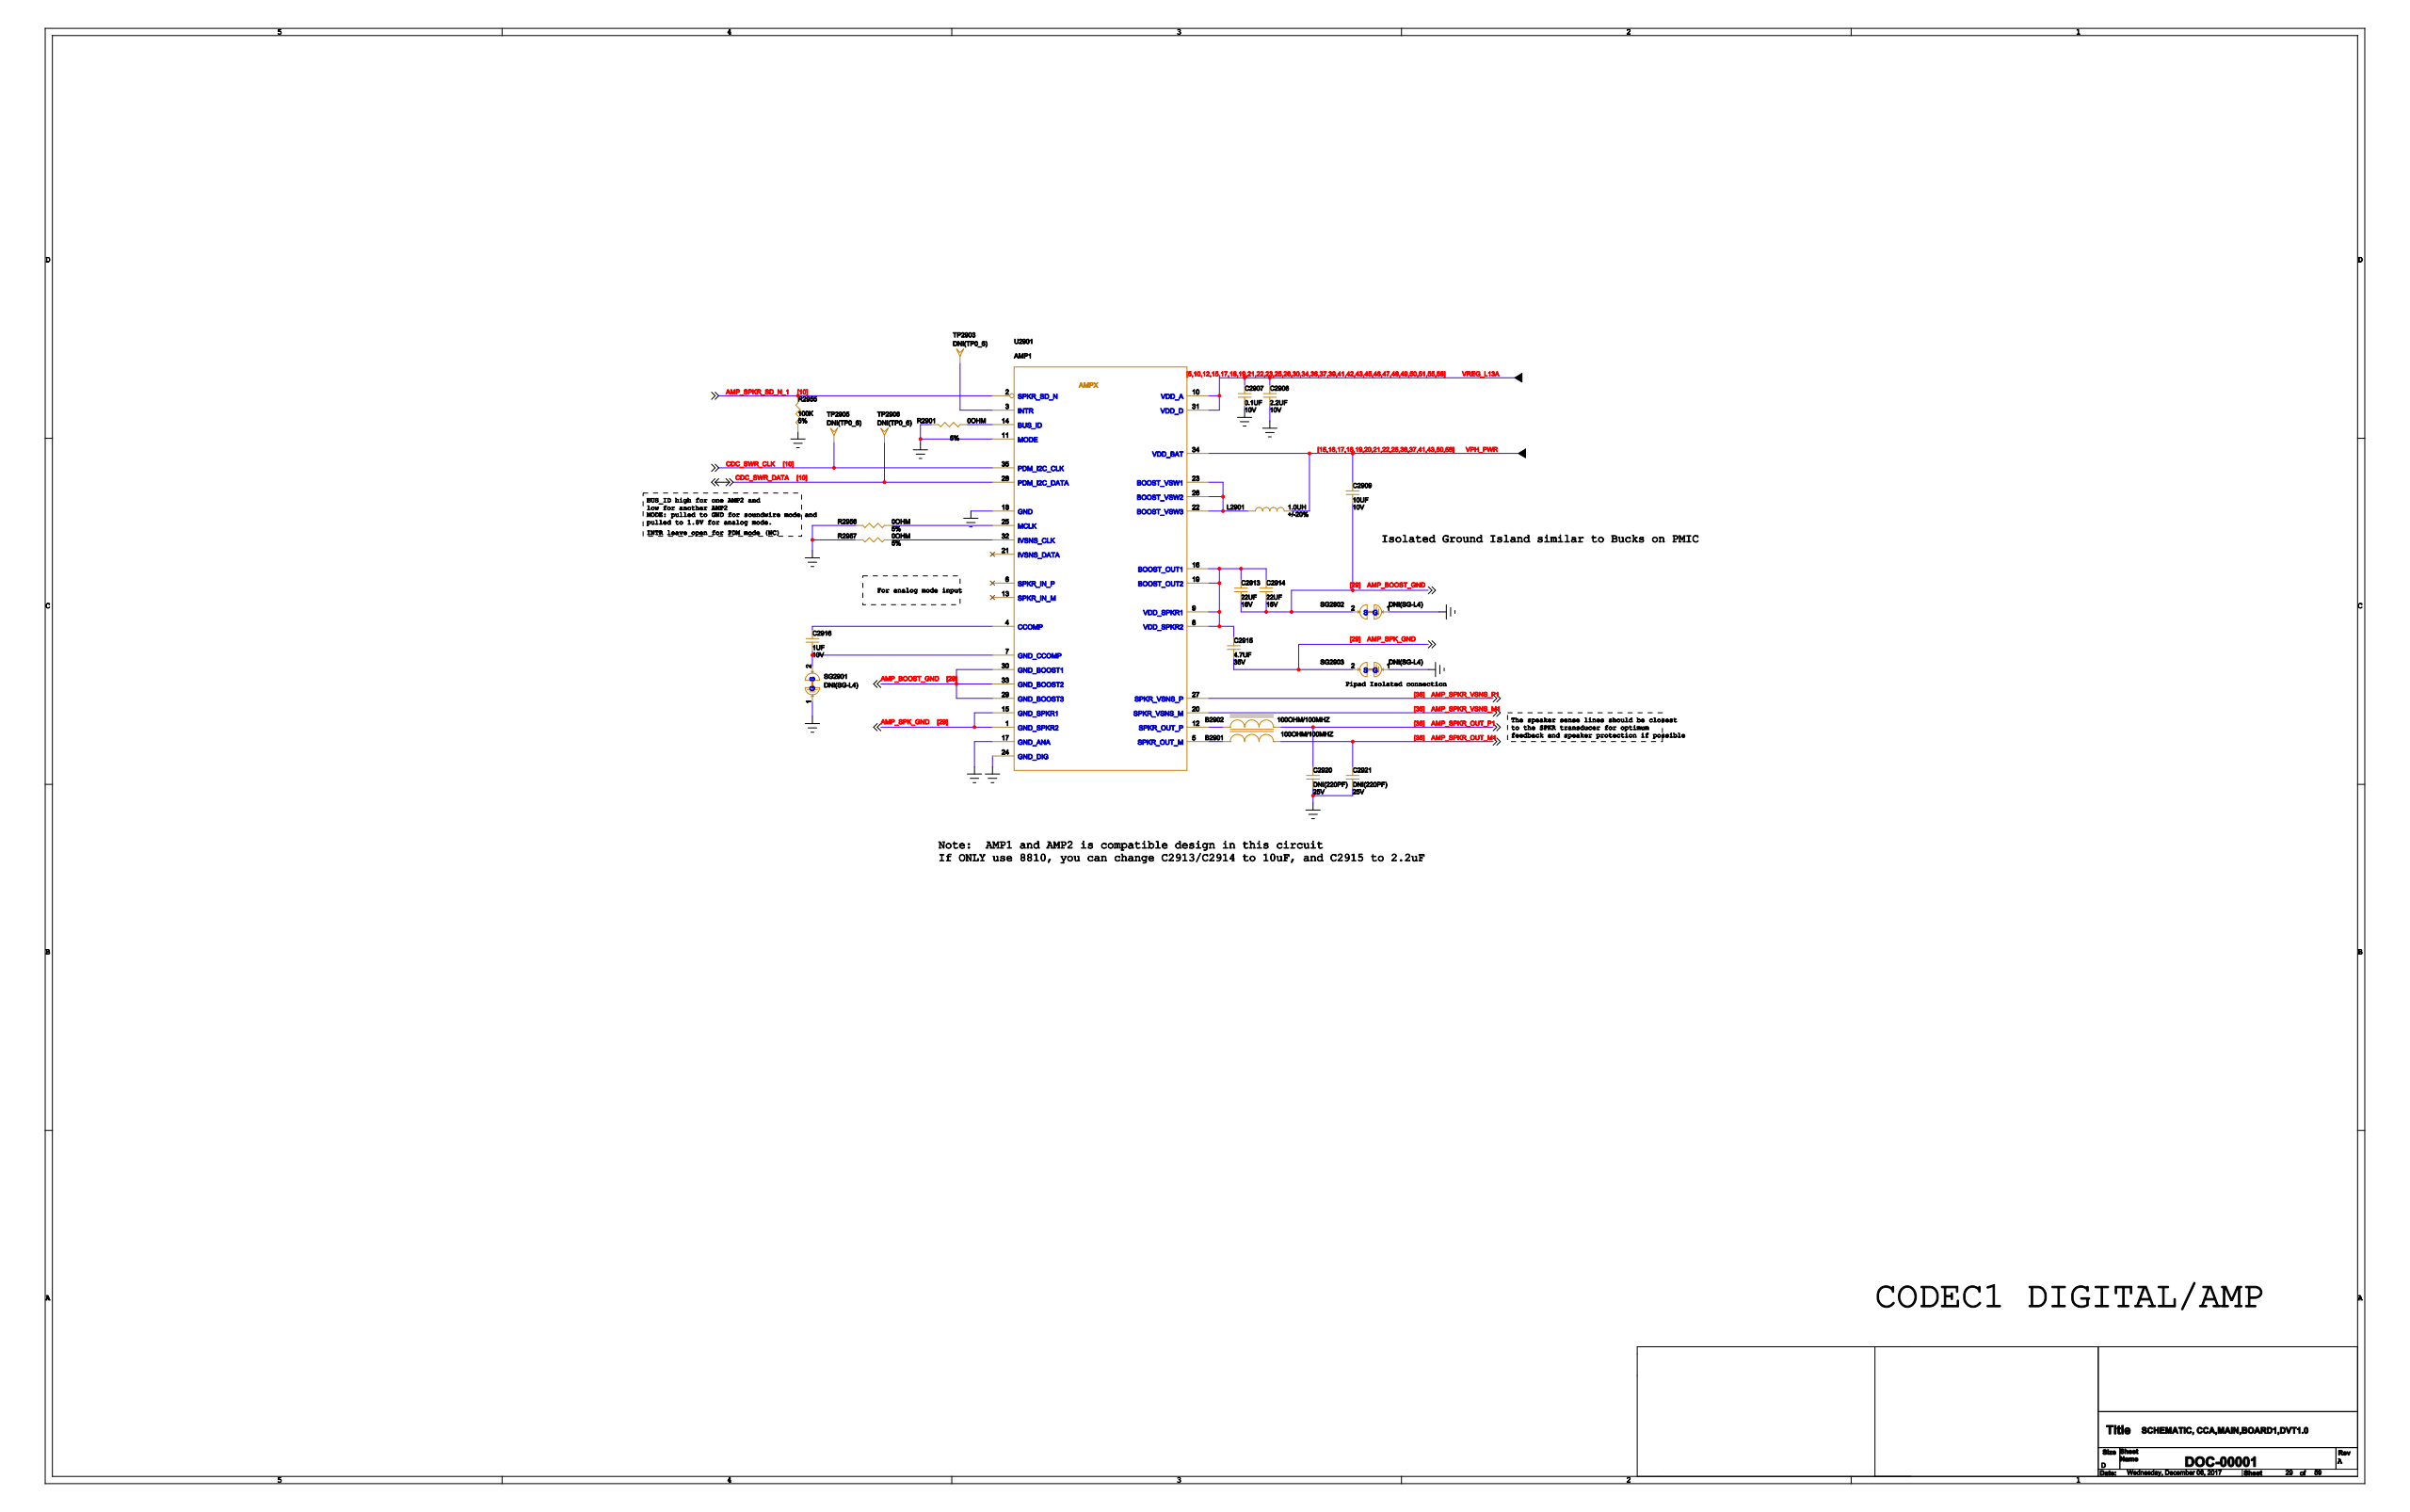Circuit board | KiCad | 1657 parts | 1365 nets | one sheet of the schematic
Parts on this sheet (reference | value | footprint):
B2901
B2902
C2906
C2907
C2909
C2913
C2914
C2915
C2916
C2920
C2921
L2901
R2901
R2955
R2956
R2957
SG2901
SG2902
SG2903
TP2903
TP2905
TP2906
U2901
Nets of these parts (net: part-pin ...):
GND: C2906-2 C2907-2 C2920-2 C2921-2 R2901-1 R2955-2 R2956-1 R2957-1 SG2901-1 SG2902-1 SG2903-1 U2901-11 U2901-17 U2901-18 U2901-24
VREG_L13A: C2906-1 C2907-1 U2901-10 U2901-31
N21625173: L2901-1 U2901-22 U2901-23 U2901-26
VPH_PWR: C2909-1 L2901-2 U2901-34
MP_SPKR_OUT_P1: B2902-2 C2920-1
N21625063: C2916-2 SG2901-2 U2901-7
AMP_BOOST_GND: C2909-2 C2913-2 C2914-2 SG2902-2 U2901-29 U2901-30 U2901-33
N21625233: B2901-1 U2901-5
MP_SPKR_OUT_M1: B2901-2 C2921-1
CDC_SWR_DATA: TP2906-1 U2901-28
AMP_SPK_GND: C2915-2 SG2903-2 U2901-1 U2901-15
N21625131: TP2903-1 U2901-3
N21625283: R2901-2 U2901-14
N21625245: C2916-1 U2901-4
MP_SPKR_SD_N_1: R2955-1 U2901-2
N21625057: C2913-1 C2914-1 C2915-1 U2901-8 U2901-9 U2901-16 U2901-19
N21625231: B2902-1 U2901-12
N21625275: R2956-2 U2901-25
N21625277: R2957-2 U2901-32
CDC_SWR_CLK: TP2905-1 U2901-35